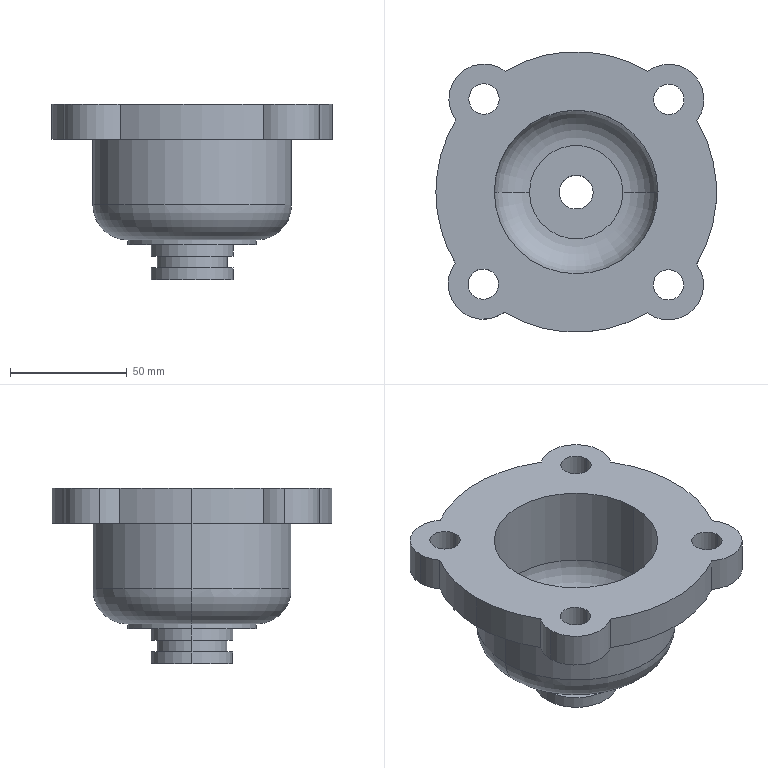Part | SolidWorks | features ICE 4, Fillet 2, Extrusion 1, Revolution 1 | 1 solid | 56 faces | box 120 x 120 x 75 mm | volume 236735 mm3 | cylinder 41 | plane 11 | torus 4 | commonest cylinder face diameters 13 x8 26 x8 30 x8 120 x5 35 x4 14.5 x2